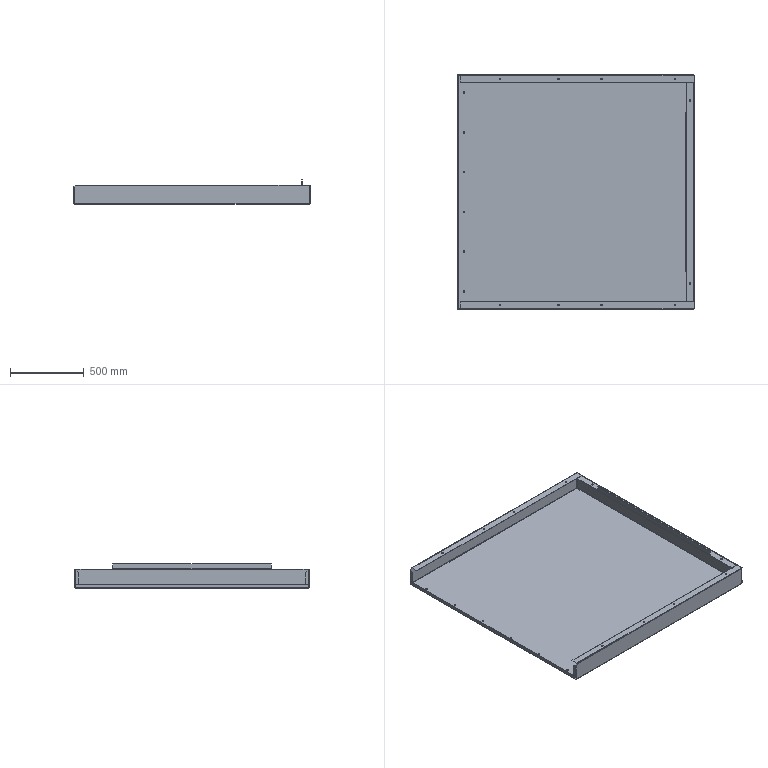Part | STEP file | SYL_0392D6J1SYL0380DJ100-232734 | 1 solid | 172 faces | box 1604 x 1592 x 165 mm | volume 6912474 mm3 | plane 120 | cylinder 52 | commonest cylinder face diameters 10.5 x20 11 x12 4 x8 8 x8 2 x2 6 x2